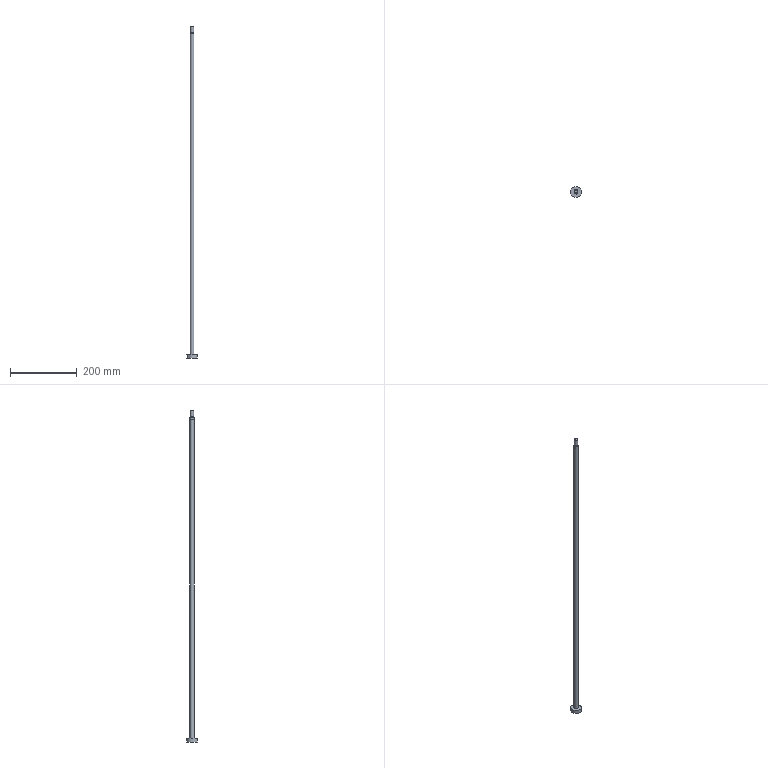Part | STEP file | 160884 CRDNG-32-400-PPV-A---(KS) | 1 solid | 19 faces | box 32 x 32 x 991.817 mm | volume 118704 mm3 | plane 9 | cylinder 4 | cone 4 | torus 2 | commonest cylinder face diameters 9.4 x1 10 x1 12 x1 32 x1
STEP:
#1=CARTESIAN_POINT('',(0.,0.,0.));
#2=DIRECTION('',(0.,0.,1.));
#3=DIRECTION('',(1.,0.,0.));
#4=AXIS2_PLACEMENT_3D('',#1,#2,#3);
#5=CARTESIAN_POINT('',(0.,4.7,226.3));
#6=VERTEX_POINT('',#5);
#7=CARTESIAN_POINT('',(4.7,0.,226.3));
#8=VERTEX_POINT('',#7);
#9=CARTESIAN_POINT('',(0.,0.,226.3));
#10=DIRECTION('',(0.,0.,1.));
#11=DIRECTION('',(0.,1.,0.));
#12=AXIS2_PLACEMENT_3D('',#9,#10,#11);
#13=CIRCLE('',#12,4.7);
#14=CARTESIAN_POINT('',(0.,0.,226.3));
#15=DIRECTION('',(0.,0.,1.));
#16=DIRECTION('',(1.,0.,0.));
#17=AXIS2_PLACEMENT_3D('',#14,#15,#16);
#18=TOROIDAL_SURFACE('',#17,5.,0.3);
#19=CARTESIAN_POINT('',(1.571,3.142));
#20=DIRECTION('',(1.,0.));
#21=VECTOR('',#20,1.);
#22=LINE('',#19,#21);
#23=(GEOMETRIC_REPRESENTATION_CONTEXT(2)PARAMETRIC_REPRESENTATION_CONTEXT()REPRESENTATION_CONTEXT('',''));
#24=DEFINITIONAL_REPRESENTATION('',(#22),#23);
#25=PCURVE('',#18,#24);
#26=CARTESIAN_POINT('',(0.,0.,226.611));
#27=DIRECTION('',(0.,0.,1.));
#28=DIRECTION('',(0.,1.,0.));
#29=AXIS2_PLACEMENT_3D('',#26,#27,#28);
#30=CYLINDRICAL_SURFACE('',#29,4.7);
#31=CARTESIAN_POINT('',(0.,-0.3105));
#32=DIRECTION('',(1.,0.));
#33=VECTOR('',#32,1.);
#34=LINE('',#31,#33);
#35=(GEOMETRIC_REPRESENTATION_CONTEXT(2)PARAMETRIC_REPRESENTATION_CONTEXT()REPRESENTATION_CONTEXT('',''));
#36=DEFINITIONAL_REPRESENTATION('',(#34),#35);
#37=PCURVE('',#30,#36);
#38=SURFACE_CURVE('',#13,(#25,#37),.PCURVE_S1.);
#39=EDGE_CURVE('',#6,#8,#38,.T.);
#40=ORIENTED_EDGE('',*,*,#39,.T.);
#41=CARTESIAN_POINT('',(5.,0.,226.));
#42=VERTEX_POINT('',#41);
#43=CARTESIAN_POINT('',(4.7,0.,226.3));
#44=CARTESIAN_POINT('',(4.7,0.,226.22));
#45=CARTESIAN_POINT('',(4.726,0.,226.142));
#46=CARTESIAN_POINT('',(4.774,0.,226.074));
#47=CARTESIAN_POINT('',(4.842,0.,226.026));
#48=CARTESIAN_POINT('',(4.92,0.,226.));
#49=CARTESIAN_POINT('',(5.,0.,226.));
#50=(BOUNDED_CURVE()B_SPLINE_CURVE(6,(#43,#44,#45,#46,#47,#48,#49),.UNSPECIFIED.,.F.,.F.)B_SPLINE_CURVE_WITH_KNOTS((7,7),(3.142,4.712),.PIECEWISE_BEZIER_KNOTS.)CURVE()GEOMETRIC_REPRESENTATION_ITEM()RATIONAL_B_SPLINE_CURVE((1.031,1.01,0.9979,0.994,0.9979,1.01,1.031))REPRESENTATION_ITEM(''));
#51=CARTESIAN_POINT('',(6.283,0.));
#52=DIRECTION('',(0.,1.));
#53=VECTOR('',#52,1.);
#54=LINE('',#51,#53);
#55=(GEOMETRIC_REPRESENTATION_CONTEXT(2)PARAMETRIC_REPRESENTATION_CONTEXT()REPRESENTATION_CONTEXT('',''));
#56=DEFINITIONAL_REPRESENTATION('',(#54),#55);
#57=PCURVE('',#18,#56);
#58=CARTESIAN_POINT('',(0.,0.));
#59=DIRECTION('',(0.,1.));
#60=VECTOR('',#59,1.);
#61=LINE('',#58,#60);
#62=(GEOMETRIC_REPRESENTATION_CONTEXT(2)PARAMETRIC_REPRESENTATION_CONTEXT()REPRESENTATION_CONTEXT('',''));
#63=DEFINITIONAL_REPRESENTATION('',(#61),#62);
#64=PCURVE('',#18,#63);
#65=SEAM_CURVE('',#50,(#57,#64),.PCURVE_S1.);
#66=EDGE_CURVE('',#8,#42,#65,.T.);
#67=ORIENTED_EDGE('',*,*,#66,.T.);
#68=CARTESIAN_POINT('',(-5.,0.,226.));
#69=VERTEX_POINT('',#68);
#70=CARTESIAN_POINT('',(0.,0.,226.));
#71=DIRECTION('',(0.,0.,1.));
#72=DIRECTION('',(1.,0.,0.));
#73=AXIS2_PLACEMENT_3D('',#70,#71,#72);
#74=CIRCLE('',#73,5.);
#75=CARTESIAN_POINT('',(0.,4.712));
#76=DIRECTION('',(1.,0.));
#77=VECTOR('',#76,1.);
#78=LINE('',#75,#77);
#79=(GEOMETRIC_REPRESENTATION_CONTEXT(2)PARAMETRIC_REPRESENTATION_CONTEXT()REPRESENTATION_CONTEXT('',''));
#80=DEFINITIONAL_REPRESENTATION('',(#78),#79);
#81=PCURVE('',#18,#80);
#82=CARTESIAN_POINT('',(0.,2.75,226.));
#83=DIRECTION('',(0.,0.,1.));
#84=DIRECTION('',(1.,0.,0.));
#85=AXIS2_PLACEMENT_3D('',#82,#83,#84);
#86=PLANE('',#85);
#87=CARTESIAN_POINT('',(0.,-2.75));
#88=DIRECTION('',(1.,0.));
#89=AXIS2_PLACEMENT_2D('',#87,#88);
#90=CIRCLE('',#89,5.);
#91=(GEOMETRIC_REPRESENTATION_CONTEXT(2)PARAMETRIC_REPRESENTATION_CONTEXT()REPRESENTATION_CONTEXT('',''));
#92=DEFINITIONAL_REPRESENTATION('',(#90),#91);
#93=PCURVE('',#86,#92);
#94=SURFACE_CURVE('',#74,(#81,#93),.PCURVE_S1.);
#95=EDGE_CURVE('',#69,#42,#94,.T.);
#96=ORIENTED_EDGE('',*,*,#95,.F.);
#97=CARTESIAN_POINT('',(0.,0.,226.));
#98=DIRECTION('',(0.,0.,1.));
#99=DIRECTION('',(1.,0.,0.));
#100=AXIS2_PLACEMENT_3D('',#97,#98,#99);
#101=CIRCLE('',#100,5.);
#102=CARTESIAN_POINT('',(0.,4.712));
#103=DIRECTION('',(1.,0.));
#104=VECTOR('',#103,1.);
#105=LINE('',#102,#104);
#106=(GEOMETRIC_REPRESENTATION_CONTEXT(2)PARAMETRIC_REPRESENTATION_CONTEXT()REPRESENTATION_CONTEXT('',''));
#107=DEFINITIONAL_REPRESENTATION('',(#105),#106);
#108=PCURVE('',#18,#107);
#109=CARTESIAN_POINT('',(0.,2.75,226.));
#110=DIRECTION('',(0.,0.,1.));
#111=DIRECTION('',(1.,0.,0.));
#112=AXIS2_PLACEMENT_3D('',#109,#110,#111);
#113=PLANE('',#112);
#114=CARTESIAN_POINT('',(0.,-2.75));
#115=DIRECTION('',(1.,0.));
#116=AXIS2_PLACEMENT_2D('',#114,#115);
#117=CIRCLE('',#116,5.);
#118=(GEOMETRIC_REPRESENTATION_CONTEXT(2)PARAMETRIC_REPRESENTATION_CONTEXT()REPRESENTATION_CONTEXT('',''));
#119=DEFINITIONAL_REPRESENTATION('',(#117),#118);
#120=PCURVE('',#113,#119);
#121=SURFACE_CURVE('',#101,(#108,#120),.PCURVE_S1.);
#122=EDGE_CURVE('',#42,#69,#121,.T.);
#123=ORIENTED_EDGE('',*,*,#122,.F.);
#124=ORIENTED_EDGE('',*,*,#66,.F.);
#125=CARTESIAN_POINT('',(0.,0.,226.3));
#126=DIRECTION('',(0.,0.,1.));
#127=DIRECTION('',(0.,1.,0.));
#128=AXIS2_PLACEMENT_3D('',#125,#126,#127);
#129=CIRCLE('',#128,4.7);
#130=CARTESIAN_POINT('',(-4.712,3.142));
#131=DIRECTION('',(1.,0.));
#132=VECTOR('',#131,1.);
#133=LINE('',#130,#132);
#134=(GEOMETRIC_REPRESENTATION_CONTEXT(2)PARAMETRIC_REPRESENTATION_CONTEXT()REPRESENTATION_CONTEXT('',''));
#135=DEFINITIONAL_REPRESENTATION('',(#133),#134);
#136=PCURVE('',#18,#135);
#137=CARTESIAN_POINT('',(0.,-0.3105));
#138=DIRECTION('',(1.,0.));
#139=VECTOR('',#138,1.);
#140=LINE('',#137,#139);
#141=(GEOMETRIC_REPRESENTATION_CONTEXT(2)PARAMETRIC_REPRESENTATION_CONTEXT()REPRESENTATION_CONTEXT('',''));
#142=DEFINITIONAL_REPRESENTATION('',(#140),#141);
#143=PCURVE('',#30,#142);
#144=SURFACE_CURVE('',#129,(#136,#143),.PCURVE_S1.);
#145=EDGE_CURVE('',#8,#6,#144,.T.);
#146=ORIENTED_EDGE('',*,*,#145,.T.);
#147=EDGE_LOOP('',(#40,#67,#96,#123,#124,#146));
#148=FACE_BOUND('',#147,.F.);
#149=ADVANCED_FACE('',(#148),#18,.F.);
#150=CARTESIAN_POINT('',(0.,4.7,226.921));
#151=VERTEX_POINT('',#150);
#152=CARTESIAN_POINT('',(0.,0.,226.921));
#153=DIRECTION('',(0.,0.,1.));
#154=DIRECTION('',(0.,1.,0.));
#155=AXIS2_PLACEMENT_3D('',#152,#153,#154);
#156=CIRCLE('',#155,4.7);
#157=CARTESIAN_POINT('',(0.,0.3105));
#158=DIRECTION('',(1.,0.));
#159=VECTOR('',#158,1.);
#160=LINE('',#157,#159);
#161=(GEOMETRIC_REPRESENTATION_CONTEXT(2)PARAMETRIC_REPRESENTATION_CONTEXT()REPRESENTATION_CONTEXT('',''));
#162=DEFINITIONAL_REPRESENTATION('',(#160),#161);
#163=PCURVE('',#30,#162);
#164=CARTESIAN_POINT('',(0.,0.,226.921));
#165=DIRECTION('',(0.,0.,1.));
#166=DIRECTION('',(1.,0.,0.));
#167=AXIS2_PLACEMENT_3D('',#164,#165,#166);
#168=TOROIDAL_SURFACE('',#167,5.3,0.6);
#169=CARTESIAN_POINT('',(1.571,9.425));
#170=DIRECTION('',(1.,0.));
#171=VECTOR('',#170,1.);
#172=LINE('',#169,#171);
#173=(GEOMETRIC_REPRESENTATION_CONTEXT(2)PARAMETRIC_REPRESENTATION_CONTEXT()REPRESENTATION_CONTEXT('',''));
#174=DEFINITIONAL_REPRESENTATION('',(#172),#173);
#175=PCURVE('',#168,#174);
#176=SURFACE_CURVE('',#156,(#163,#175),.PCURVE_S1.);
#177=EDGE_CURVE('',#151,#151,#176,.T.);
#178=ORIENTED_EDGE('',*,*,#177,.F.);
#179=CARTESIAN_POINT('',(0.,4.7,226.3));
#180=CARTESIAN_POINT('',(0.,4.7,226.921));
#181=B_SPLINE_CURVE_WITH_KNOTS('',1,(#179,#180),.UNSPECIFIED.,.F.,.F.,(2,2),(-0.3105,0.3105),.PIECEWISE_BEZIER_KNOTS.);
#182=CARTESIAN_POINT('',(0.,0.));
#183=DIRECTION('',(0.,1.));
#184=VECTOR('',#183,1.);
#185=LINE('',#182,#184);
#186=(GEOMETRIC_REPRESENTATION_CONTEXT(2)PARAMETRIC_REPRESENTATION_CONTEXT()REPRESENTATION_CONTEXT('',''));
#187=DEFINITIONAL_REPRESENTATION('',(#185),#186);
#188=PCURVE('',#30,#187);
#189=CARTESIAN_POINT('',(6.283,0.));
#190=DIRECTION('',(0.,1.));
#191=VECTOR('',#190,1.);
#192=LINE('',#189,#191);
#193=(GEOMETRIC_REPRESENTATION_CONTEXT(2)PARAMETRIC_REPRESENTATION_CONTEXT()REPRESENTATION_CONTEXT('',''));
#194=DEFINITIONAL_REPRESENTATION('',(#192),#193);
#195=PCURVE('',#30,#194);
#196=SEAM_CURVE('',#181,(#188,#195),.PCURVE_S1.);
#197=EDGE_CURVE('',#6,#151,#196,.T.);
#198=ORIENTED_EDGE('',*,*,#197,.F.);
#199=ORIENTED_EDGE('',*,*,#39,.T.);
#200=ORIENTED_EDGE('',*,*,#145,.T.);
#201=ORIENTED_EDGE('',*,*,#197,.T.);
#202=EDGE_LOOP('',(#178,#198,#199,#200,#201));
#203=FACE_BOUND('',#202,.T.);
#204=ADVANCED_FACE('',(#203),#30,.T.);
#205=CARTESIAN_POINT('',(0.,4.72,227.076));
#206=VERTEX_POINT('',#205);
#207=CARTESIAN_POINT('',(0.,0.,227.076));
#208=DIRECTION('',(0.,0.,1.));
#209=DIRECTION('',(0.,1.,0.));
#210=AXIS2_PLACEMENT_3D('',#207,#208,#209);
#211=CIRCLE('',#210,4.72);
#212=CARTESIAN_POINT('',(1.571,9.163));
#213=DIRECTION('',(1.,0.));
#214=VECTOR('',#213,1.);
#215=LINE('',#212,#214);
#216=(GEOMETRIC_REPRESENTATION_CONTEXT(2)PARAMETRIC_REPRESENTATION_CONTEXT()REPRESENTATION_CONTEXT('',''));
#217=DEFINITIONAL_REPRESENTATION('',(#215),#216);
#218=PCURVE('',#168,#217);
#219=CARTESIAN_POINT('',(0.,0.,227.598));
#220=DIRECTION('',(0.,0.,1.));
#221=DIRECTION('',(0.,1.,0.));
#222=AXIS2_PLACEMENT_3D('',#219,#220,#221);
#223=CONICAL_SURFACE('',#222,4.86,0.2618);
#224=CARTESIAN_POINT('',(0.,-0.5217));
#225=DIRECTION('',(1.,0.));
#226=VECTOR('',#225,1.);
#227=LINE('',#224,#226);
#228=(GEOMETRIC_REPRESENTATION_CONTEXT(2)PARAMETRIC_REPRESENTATION_CONTEXT()REPRESENTATION_CONTEXT('',''));
#229=DEFINITIONAL_REPRESENTATION('',(#227),#228);
#230=PCURVE('',#223,#229);
#231=SURFACE_CURVE('',#211,(#218,#230),.PCURVE_S1.);
#232=EDGE_CURVE('',#206,#206,#231,.T.);
#233=ORIENTED_EDGE('',*,*,#232,.T.);
#234=CARTESIAN_POINT('',(0.,4.72,227.076));
#235=CARTESIAN_POINT('',(0.,4.714,227.051));
#236=CARTESIAN_POINT('',(0.,4.708,227.025));
#237=CARTESIAN_POINT('',(0.,4.704,226.999));
#238=CARTESIAN_POINT('',(0.,4.701,226.973));
#239=CARTESIAN_POINT('',(0.,4.7,226.947));
#240=CARTESIAN_POINT('',(0.,4.7,226.921));
#241=(BOUNDED_CURVE()B_SPLINE_CURVE(6,(#234,#235,#236,#237,#238,#239,#240),.UNSPECIFIED.,.F.,.F.)B_SPLINE_CURVE_WITH_KNOTS((7,7),(2.88,3.142),.PIECEWISE_BEZIER_KNOTS.)CURVE()GEOMETRIC_REPRESENTATION_ITEM()RATIONAL_B_SPLINE_CURVE((1.001,1.,0.9999,0.9998,0.9999,1.,1.001))REPRESENTATION_ITEM(''));
#242=CARTESIAN_POINT('',(7.854,6.283));
#243=DIRECTION('',(0.,1.));
#244=VECTOR('',#243,1.);
#245=LINE('',#242,#244);
#246=(GEOMETRIC_REPRESENTATION_CONTEXT(2)PARAMETRIC_REPRESENTATION_CONTEXT()REPRESENTATION_CONTEXT('',''));
#247=DEFINITIONAL_REPRESENTATION('',(#245),#246);
#248=PCURVE('',#168,#247);
#249=CARTESIAN_POINT('',(1.571,6.283));
#250=DIRECTION('',(0.,1.));
#251=VECTOR('',#250,1.);
#252=LINE('',#249,#251);
#253=(GEOMETRIC_REPRESENTATION_CONTEXT(2)PARAMETRIC_REPRESENTATION_CONTEXT()REPRESENTATION_CONTEXT('',''));
#254=DEFINITIONAL_REPRESENTATION('',(#252),#253);
#255=PCURVE('',#168,#254);
#256=SEAM_CURVE('',#241,(#248,#255),.PCURVE_S1.);
#257=EDGE_CURVE('',#206,#151,#256,.T.);
#258=ORIENTED_EDGE('',*,*,#257,.T.);
#259=ORIENTED_EDGE('',*,*,#177,.F.);
#260=ORIENTED_EDGE('',*,*,#257,.F.);
#261=EDGE_LOOP('',(#233,#258,#259,#260));
#262=FACE_BOUND('',#261,.F.);
#263=ADVANCED_FACE('',(#262),#168,.F.);
#264=CARTESIAN_POINT('',(0.,5.,228.12));
#265=VERTEX_POINT('',#264);
#266=CARTESIAN_POINT('',(0.,0.,228.12));
#267=DIRECTION('',(0.,0.,1.));
#268=DIRECTION('',(0.,1.,0.));
#269=AXIS2_PLACEMENT_3D('',#266,#267,#268);
#270=CIRCLE('',#269,5.);
#271=CARTESIAN_POINT('',(0.,0.5217));
#272=DIRECTION('',(1.,0.));
#273=VECTOR('',#272,1.);
#274=LINE('',#271,#273);
#275=(GEOMETRIC_REPRESENTATION_CONTEXT(2)PARAMETRIC_REPRESENTATION_CONTEXT()REPRESENTATION_CONTEXT('',''));
#276=DEFINITIONAL_REPRESENTATION('',(#274),#275);
#277=PCURVE('',#223,#276);
#278=CARTESIAN_POINT('',(0.,0.,237.676));
#279=DIRECTION('',(0.,0.,1.));
#280=DIRECTION('',(0.,1.,0.));
#281=AXIS2_PLACEMENT_3D('',#278,#279,#280);
#282=CYLINDRICAL_SURFACE('',#281,5.);
#283=CARTESIAN_POINT('',(0.,-9.557));
#284=DIRECTION('',(1.,0.));
#285=VECTOR('',#284,1.);
#286=LINE('',#283,#285);
#287=(GEOMETRIC_REPRESENTATION_CONTEXT(2)PARAMETRIC_REPRESENTATION_CONTEXT()REPRESENTATION_CONTEXT('',''));
#288=DEFINITIONAL_REPRESENTATION('',(#286),#287);
#289=PCURVE('',#282,#288);
#290=SURFACE_CURVE('',#270,(#277,#289),.PCURVE_S1.);
#291=EDGE_CURVE('',#265,#265,#290,.T.);
#292=ORIENTED_EDGE('',*,*,#291,.F.);
#293=CARTESIAN_POINT('',(0.,4.72,227.076));
#294=CARTESIAN_POINT('',(0.,5.,228.12));
#295=B_SPLINE_CURVE_WITH_KNOTS('',1,(#293,#294),.UNSPECIFIED.,.F.,.F.,(2,2),(-0.5401,0.5401),.PIECEWISE_BEZIER_KNOTS.);
#296=CARTESIAN_POINT('',(0.,0.));
#297=DIRECTION('',(0.,1.));
#298=VECTOR('',#297,1.);
#299=LINE('',#296,#298);
#300=(GEOMETRIC_REPRESENTATION_CONTEXT(2)PARAMETRIC_REPRESENTATION_CONTEXT()REPRESENTATION_CONTEXT('',''));
#301=DEFINITIONAL_REPRESENTATION('',(#299),#300);
#302=PCURVE('',#223,#301);
#303=CARTESIAN_POINT('',(6.283,0.));
#304=DIRECTION('',(0.,1.));
#305=VECTOR('',#304,1.);
#306=LINE('',#303,#305);
#307=(GEOMETRIC_REPRESENTATION_CONTEXT(2)PARAMETRIC_REPRESENTATION_CONTEXT()REPRESENTATION_CONTEXT('',''));
#308=DEFINITIONAL_REPRESENTATION('',(#306),#307);
#309=PCURVE('',#223,#308);
#310=SEAM_CURVE('',#295,(#302,#309),.PCURVE_S1.);
#311=EDGE_CURVE('',#206,#265,#310,.T.);
#312=ORIENTED_EDGE('',*,*,#311,.F.);
#313=ORIENTED_EDGE('',*,*,#232,.T.);
#314=ORIENTED_EDGE('',*,*,#311,.T.);
#315=EDGE_LOOP('',(#292,#312,#313,#314));
#316=FACE_BOUND('',#315,.T.);
#317=ADVANCED_FACE('',(#316),#223,.T.);
#318=CARTESIAN_POINT('',(0.,5.,247.233));
#319=VERTEX_POINT('',#318);
#320=CARTESIAN_POINT('',(0.,0.,247.233));
#321=DIRECTION('',(0.,0.,1.));
#322=DIRECTION('',(0.,1.,0.));
#323=AXIS2_PLACEMENT_3D('',#320,#321,#322);
#324=CIRCLE('',#323,5.);
#325=CARTESIAN_POINT('',(0.,9.557));
#326=DIRECTION('',(1.,0.));
#327=VECTOR('',#326,1.);
#328=LINE('',#325,#327);
#329=(GEOMETRIC_REPRESENTATION_CONTEXT(2)PARAMETRIC_REPRESENTATION_CONTEXT()REPRESENTATION_CONTEXT('',''));
#330=DEFINITIONAL_REPRESENTATION('',(#328),#329);
#331=PCURVE('',#282,#330);
#332=CARTESIAN_POINT('',(0.,0.,247.617));
#333=DIRECTION('',(0.,0.,-1.));
#334=DIRECTION('',(0.,1.,0.));
#335=AXIS2_PLACEMENT_3D('',#332,#333,#334);
#336=CONICAL_SURFACE('',#335,4.617,0.7854);
#337=CARTESIAN_POINT('',(6.283,0.3835));
#338=DIRECTION('',(-1.,0.));
#339=VECTOR('',#338,1.);
#340=LINE('',#337,#339);
#341=(GEOMETRIC_REPRESENTATION_CONTEXT(2)PARAMETRIC_REPRESENTATION_CONTEXT()REPRESENTATION_CONTEXT('',''));
#342=DEFINITIONAL_REPRESENTATION('',(#340),#341);
#343=PCURVE('',#336,#342);
#344=SURFACE_CURVE('',#324,(#331,#343),.PCURVE_S1.);
#345=EDGE_CURVE('',#319,#319,#344,.T.);
#346=ORIENTED_EDGE('',*,*,#345,.F.);
#347=CARTESIAN_POINT('',(0.,5.,228.12));
#348=CARTESIAN_POINT('',(0.,5.,247.233));
#349=B_SPLINE_CURVE_WITH_KNOTS('',1,(#347,#348),.UNSPECIFIED.,.F.,.F.,(2,2),(-9.557,9.557),.PIECEWISE_BEZIER_KNOTS.);
#350=CARTESIAN_POINT('',(0.,0.));
#351=DIRECTION('',(0.,1.));
#352=VECTOR('',#351,1.);
#353=LINE('',#350,#352);
#354=(GEOMETRIC_REPRESENTATION_CONTEXT(2)PARAMETRIC_REPRESENTATION_CONTEXT()REPRESENTATION_CONTEXT('',''));
#355=DEFINITIONAL_REPRESENTATION('',(#353),#354);
#356=PCURVE('',#282,#355);
#357=CARTESIAN_POINT('',(6.283,0.));
#358=DIRECTION('',(0.,1.));
#359=VECTOR('',#358,1.);
#360=LINE('',#357,#359);
#361=(GEOMETRIC_REPRESENTATION_CONTEXT(2)PARAMETRIC_REPRESENTATION_CONTEXT()REPRESENTATION_CONTEXT('',''));
#362=DEFINITIONAL_REPRESENTATION('',(#360),#361);
#363=PCURVE('',#282,#362);
#364=SEAM_CURVE('',#349,(#356,#363),.PCURVE_S1.);
#365=EDGE_CURVE('',#265,#319,#364,.T.);
#366=ORIENTED_EDGE('',*,*,#365,.F.);
#367=ORIENTED_EDGE('',*,*,#291,.T.);
#368=ORIENTED_EDGE('',*,*,#365,.T.);
#369=EDGE_LOOP('',(#346,#366,#367,#368));
#370=FACE_BOUND('',#369,.T.);
#371=ADVANCED_FACE('',(#370),#282,.T.);
#372=CARTESIAN_POINT('',(0.,4.233,248.));
#373=VERTEX_POINT('',#372);
#374=CARTESIAN_POINT('',(0.,0.,248.));
#375=DIRECTION('',(0.,0.,1.));
#376=DIRECTION('',(0.,1.,0.));
#377=AXIS2_PLACEMENT_3D('',#374,#375,#376);
#378=CIRCLE('',#377,4.233);
#379=CARTESIAN_POINT('',(6.283,-0.3835));
#380=DIRECTION('',(-1.,0.));
#381=VECTOR('',#380,1.);
#382=LINE('',#379,#381);
#383=(GEOMETRIC_REPRESENTATION_CONTEXT(2)PARAMETRIC_REPRESENTATION_CONTEXT()REPRESENTATION_CONTEXT('',''));
#384=DEFINITIONAL_REPRESENTATION('',(#382),#383);
#385=PCURVE('',#336,#384);
#386=CARTESIAN_POINT('',(0.,2.116,248.));
#387=DIRECTION('',(0.,0.,1.));
#388=DIRECTION('',(1.,0.,0.));
#389=AXIS2_PLACEMENT_3D('',#386,#387,#388);
#390=PLANE('',#389);
#391=CARTESIAN_POINT('',(0.,-2.116));
#392=DIRECTION('',(0.,1.));
#393=AXIS2_PLACEMENT_2D('',#391,#392);
#394=CIRCLE('',#393,4.233);
#395=(GEOMETRIC_REPRESENTATION_CONTEXT(2)PARAMETRIC_REPRESENTATION_CONTEXT()REPRESENTATION_CONTEXT('',''));
#396=DEFINITIONAL_REPRESENTATION('',(#394),#395);
#397=PCURVE('',#390,#396);
#398=SURFACE_CURVE('',#378,(#385,#397),.PCURVE_S1.);
#399=EDGE_CURVE('',#373,#373,#398,.T.);
#400=ORIENTED_EDGE('',*,*,#399,.F.);
#401=CARTESIAN_POINT('',(0.,4.233,248.));
#402=CARTESIAN_POINT('',(0.,5.,247.233));
#403=B_SPLINE_CURVE_WITH_KNOTS('',1,(#401,#402),.UNSPECIFIED.,.F.,.F.,(2,2),(-0.5424,0.5424),.PIECEWISE_BEZIER_KNOTS.);
#404=CARTESIAN_POINT('',(6.283,0.));
#405=DIRECTION('',(0.,1.));
#406=VECTOR('',#405,1.);
#407=LINE('',#404,#406);
#408=(GEOMETRIC_REPRESENTATION_CONTEXT(2)PARAMETRIC_REPRESENTATION_CONTEXT()REPRESENTATION_CONTEXT('',''));
#409=DEFINITIONAL_REPRESENTATION('',(#407),#408);
#410=PCURVE('',#336,#409);
#411=CARTESIAN_POINT('',(0.,0.));
#412=DIRECTION('',(0.,1.));
#413=VECTOR('',#412,1.);
#414=LINE('',#411,#413);
#415=(GEOMETRIC_REPRESENTATION_CONTEXT(2)PARAMETRIC_REPRESENTATION_CONTEXT()REPRESENTATION_CONTEXT('',''));
#416=DEFINITIONAL_REPRESENTATION('',(#414),#415);
#417=PCURVE('',#336,#416);
#418=SEAM_CURVE('',#403,(#410,#417),.PCURVE_S1.);
#419=EDGE_CURVE('',#373,#319,#418,.T.);
#420=ORIENTED_EDGE('',*,*,#419,.T.);
#421=ORIENTED_EDGE('',*,*,#345,.T.);
#422=ORIENTED_EDGE('',*,*,#419,.F.);
#423=EDGE_LOOP('',(#400,#420,#421,#422));
#424=FACE_BOUND('',#423,.T.);
#425=ADVANCED_FACE('',(#424),#336,.T.);
#426=ORIENTED_EDGE('',*,*,#399,.T.);
#427=EDGE_LOOP('',(#426));
#428=FACE_BOUND('',#427,.T.);
#429=ADVANCED_FACE('',(#428),#390,.T.);
#430=ORIENTED_EDGE('',*,*,#122,.F.);
#431=CARTESIAN_POINT('',(5.,2.291,226.));
#432=VERTEX_POINT('',#431);
#433=CARTESIAN_POINT('',(5.,1.375,226.));
#434=DIRECTION('',(0.,1.,0.));
#435=VECTOR('',#434,1.);
#436=LINE('',#433,#435);
#437=CARTESIAN_POINT('',(5.,-1.375));
#438=DIRECTION('',(0.,1.));
#439=VECTOR('',#438,1.);
#440=LINE('',#437,#439);
#441=(GEOMETRIC_REPRESENTATION_CONTEXT(2)PARAMETRIC_REPRESENTATION_CONTEXT()REPRESENTATION_CONTEXT('',''));
#442=DEFINITIONAL_REPRESENTATION('',(#440),#441);
#443=PCURVE('',#113,#442);
#444=CARTESIAN_POINT('',(5.,0.,226.));
#445=DIRECTION('',(-1.,0.,0.));
#446=DIRECTION('',(0.,0.,1.));
#447=AXIS2_PLACEMENT_3D('',#444,#445,#446);
#448=PLANE('',#447);
#449=CARTESIAN_POINT('',(0.,1.375));
#450=DIRECTION('',(0.,1.));
#451=VECTOR('',#450,1.);
#452=LINE('',#449,#451);
#453=(GEOMETRIC_REPRESENTATION_CONTEXT(2)PARAMETRIC_REPRESENTATION_CONTEXT()REPRESENTATION_CONTEXT('',''));
#454=DEFINITIONAL_REPRESENTATION('',(#452),#453);
#455=PCURVE('',#448,#454);
#456=SURFACE_CURVE('',#436,(#443,#455),.PCURVE_S1.);
#457=EDGE_CURVE('',#42,#432,#456,.T.);
#458=ORIENTED_EDGE('',*,*,#457,.T.);
#459=CARTESIAN_POINT('',(-5.,2.291,226.));
#460=VERTEX_POINT('',#459);
#461=CARTESIAN_POINT('',(0.,0.,226.));
#462=DIRECTION('',(0.,0.,1.));
#463=DIRECTION('',(0.,1.,0.));
#464=AXIS2_PLACEMENT_3D('',#461,#462,#463);
#465=CIRCLE('',#464,5.5);
#466=CARTESIAN_POINT('',(0.,-2.75));
#467=DIRECTION('',(0.,1.));
#468=AXIS2_PLACEMENT_2D('',#466,#467);
#469=CIRCLE('',#468,5.5);
#470=(GEOMETRIC_REPRESENTATION_CONTEXT(2)PARAMETRIC_REPRESENTATION_CONTEXT()REPRESENTATION_CONTEXT('',''));
#471=DEFINITIONAL_REPRESENTATION('',(#469),#470);
#472=PCURVE('',#113,#471);
#473=CARTESIAN_POINT('',(0.,0.,225.75));
#474=DIRECTION('',(0.,0.,-1.));
#475=DIRECTION('',(0.,1.,0.));
#476=AXIS2_PLACEMENT_3D('',#473,#474,#475);
#477=CONICAL_SURFACE('',#476,5.75,0.7854);
#478=CARTESIAN_POINT('',(12.566,-0.25));
#479=DIRECTION('',(-1.,0.));
#480=VECTOR('',#479,1.);
#481=LINE('',#478,#480);
#482=(GEOMETRIC_REPRESENTATION_CONTEXT(2)PARAMETRIC_REPRESENTATION_CONTEXT()REPRESENTATION_CONTEXT('',''));
#483=DEFINITIONAL_REPRESENTATION('',(#481),#482);
#484=PCURVE('',#477,#483);
#485=SURFACE_CURVE('',#465,(#472,#484),.PCURVE_S1.);
#486=EDGE_CURVE('',#432,#460,#485,.T.);
#487=ORIENTED_EDGE('',*,*,#486,.T.);
#488=CARTESIAN_POINT('',(-5.,1.375,226.));
#489=DIRECTION('',(0.,-1.,0.));
#490=VECTOR('',#489,1.);
#491=LINE('',#488,#490);
#492=CARTESIAN_POINT('',(-5.,-1.375));
#493=DIRECTION('',(0.,-1.));
#494=VECTOR('',#493,1.);
#495=LINE('',#492,#494);
#496=(GEOMETRIC_REPRESENTATION_CONTEXT(2)PARAMETRIC_REPRESENTATION_CONTEXT()REPRESENTATION_CONTEXT('',''));
#497=DEFINITIONAL_REPRESENTATION('',(#495),#496);
#498=PCURVE('',#113,#497);
#499=CARTESIAN_POINT('',(-5.,0.,220.));
#500=DIRECTION('',(1.,0.,0.));
#501=DIRECTION('',(0.,0.,-1.));
#502=AXIS2_PLACEMENT_3D('',#499,#500,#501);
#503=PLANE('',#502);
#504=CARTESIAN_POINT('',(-6.,1.375));
#505=DIRECTION('',(0.,-1.));
#506=VECTOR('',#505,1.);
#507=LINE('',#504,#506);
#508=(GEOMETRIC_REPRESENTATION_CONTEXT(2)PARAMETRIC_REPRESENTATION_CONTEXT()REPRESENTATION_CONTEXT('',''));
#509=DEFINITIONAL_REPRESENTATION('',(#507),#508);
#510=PCURVE('',#503,#509);
#511=SURFACE_CURVE('',#491,(#498,#510),.PCURVE_S1.);
#512=EDGE_CURVE('',#460,#69,#511,.T.);
#513=ORIENTED_EDGE('',*,*,#512,.T.);
#514=EDGE_LOOP('',(#430,#458,#487,#513));
#515=FACE_BOUND('',#514,.T.);
#516=ADVANCED_FACE('',(#515),#113,.T.);
#517=ORIENTED_EDGE('',*,*,#95,.F.);
#518=CARTESIAN_POINT('',(-5.,-2.291,226.));
#519=VERTEX_POINT('',#518);
#520=CARTESIAN_POINT('',(-5.,1.375,226.));
#521=DIRECTION('',(0.,-1.,0.));
#522=VECTOR('',#521,1.);
#523=LINE('',#520,#522);
#524=CARTESIAN_POINT('',(-5.,-1.375));
#525=DIRECTION('',(0.,-1.));
#526=VECTOR('',#525,1.);
#527=LINE('',#524,#526);
#528=(GEOMETRIC_REPRESENTATION_CONTEXT(2)PARAMETRIC_REPRESENTATION_CONTEXT()REPRESENTATION_CONTEXT('',''));
#529=DEFINITIONAL_REPRESENTATION('',(#527),#528);
#530=PCURVE('',#86,#529);
#531=CARTESIAN_POINT('',(-6.,1.375));
#532=DIRECTION('',(0.,-1.));
#533=VECTOR('',#532,1.);
#534=LINE('',#531,#533);
#535=(GEOMETRIC_REPRESENTATION_CONTEXT(2)PARAMETRIC_REPRESENTATION_CONTEXT()REPRESENTATION_CONTEXT('',''));
#536=DEFINITIONAL_REPRESENTATION('',(#534),#535);
#537=PCURVE('',#503,#536);
#538=SURFACE_CURVE('',#523,(#530,#537),.PCURVE_S1.);
#539=EDGE_CURVE('',#69,#519,#538,.T.);
#540=ORIENTED_EDGE('',*,*,#539,.T.);
#541=CARTESIAN_POINT('',(5.,-2.291,226.));
#542=VERTEX_POINT('',#541);
#543=CARTESIAN_POINT('',(0.,0.,226.));
#544=DIRECTION('',(0.,0.,1.));
#545=DIRECTION('',(0.,1.,0.));
#546=AXIS2_PLACEMENT_3D('',#543,#544,#545);
#547=CIRCLE('',#546,5.5);
#548=CARTESIAN_POINT('',(0.,-2.75));
#549=DIRECTION('',(0.,1.));
#550=AXIS2_PLACEMENT_2D('',#548,#549);
#551=CIRCLE('',#550,5.5);
#552=(GEOMETRIC_REPRESENTATION_CONTEXT(2)PARAMETRIC_REPRESENTATION_CONTEXT()REPRESENTATION_CONTEXT('',''));
#553=DEFINITIONAL_REPRESENTATION('',(#551),#552);
#554=PCURVE('',#86,#553);
#555=CARTESIAN_POINT('',(0.,0.,225.75));
#556=DIRECTION('',(0.,0.,-1.));
#557=DIRECTION('',(0.,1.,0.));
#558=AXIS2_PLACEMENT_3D('',#555,#556,#557);
#559=CONICAL_SURFACE('',#558,5.75,0.7854);
#560=CARTESIAN_POINT('',(6.283,-0.25));
#561=DIRECTION('',(-1.,0.));
#562=VECTOR('',#561,1.);
#563=LINE('',#560,#562);
#564=(GEOMETRIC_REPRESENTATION_CONTEXT(2)PARAMETRIC_REPRESENTATION_CONTEXT()REPRESENTATION_CONTEXT('',''));
#565=DEFINITIONAL_REPRESENTATION('',(#563),#564);
#566=PCURVE('',#559,#565);
#567=SURFACE_CURVE('',#547,(#554,#566),.PCURVE_S1.);
#568=EDGE_CURVE('',#519,#542,#567,.T.);
#569=ORIENTED_EDGE('',*,*,#568,.T.);
#570=CARTESIAN_POINT('',(5.,1.375,226.));
#571=DIRECTION('',(0.,1.,0.));
#572=VECTOR('',#571,1.);
#573=LINE('',#570,#572);
#574=CARTESIAN_POINT('',(5.,-1.375));
#575=DIRECTION('',(0.,1.));
#576=VECTOR('',#575,1.);
#577=LINE('',#574,#576);
#578=(GEOMETRIC_REPRESENTATION_CONTEXT(2)PARAMETRIC_REPRESENTATION_CONTEXT()REPRESENTATION_CONTEXT('',''));
#579=DEFINITIONAL_REPRESENTATION('',(#577),#578);
#580=PCURVE('',#86,#579);
#581=CARTESIAN_POINT('',(0.,1.375));
#582=DIRECTION('',(0.,1.));
#583=VECTOR('',#582,1.);
#584=LINE('',#581,#583);
#585=(GEOMETRIC_REPRESENTATION_CONTEXT(2)PARAMETRIC_REPRESENTATION_CONTEXT()REPRESENTATION_CONTEXT('',''));
#586=DEFINITIONAL_REPRESENTATION('',(#584),#585);
#587=PCURVE('',#448,#586);
#588=SURFACE_CURVE('',#573,(#580,#587),.PCURVE_S1.);
#589=EDGE_CURVE('',#542,#42,#588,.T.);
#590=ORIENTED_EDGE('',*,*,#589,.T.);
#591=EDGE_LOOP('',(#517,#540,#569,#590));
#592=FACE_BOUND('',#591,.T.);
#593=ADVANCED_FACE('',(#592),#86,.T.);
#594=CARTESIAN_POINT('',(-5.,3.317,220.));
#595=VERTEX_POINT('',#594);
#596=CARTESIAN_POINT('',(-5.,3.317,225.5));
#597=VERTEX_POINT('',#596);
#598=CARTESIAN_POINT('',(-5.,3.317,-303.825));
#599=DIRECTION('',(0.,0.,1.));
#600=VECTOR('',#599,1.);
#601=LINE('',#598,#600);
#602=CARTESIAN_POINT('',(523.825,3.317));
#603=DIRECTION('',(-1.,0.));
#604=VECTOR('',#603,1.);
#605=LINE('',#602,#604);
#606=(GEOMETRIC_REPRESENTATION_CONTEXT(2)PARAMETRIC_REPRESENTATION_CONTEXT()REPRESENTATION_CONTEXT('',''));
#607=DEFINITIONAL_REPRESENTATION('',(#605),#606);
#608=PCURVE('',#503,#607);
#609=CARTESIAN_POINT('',(0.,0.,-303.825));
#610=DIRECTION('',(0.,0.,1.));
#611=DIRECTION('',(0.,1.,0.));
#612=AXIS2_PLACEMENT_3D('',#609,#610,#611);
#613=CYLINDRICAL_SURFACE('',#612,6.);
#614=CARTESIAN_POINT('',(7.268,0.));
#615=DIRECTION('',(0.,1.));
#616=VECTOR('',#615,1.);
#617=LINE('',#614,#616);
#618=(GEOMETRIC_REPRESENTATION_CONTEXT(2)PARAMETRIC_REPRESENTATION_CONTEXT()REPRESENTATION_CONTEXT('',''));
#619=DEFINITIONAL_REPRESENTATION('',(#617),#618);
#620=PCURVE('',#613,#619);
#621=SURFACE_CURVE('',#601,(#608,#620),.PCURVE_S1.);
#622=EDGE_CURVE('',#595,#597,#621,.T.);
#623=ORIENTED_EDGE('',*,*,#622,.F.);
#624=CARTESIAN_POINT('',(-5.,-3.317,220.));
#625=VERTEX_POINT('',#624);
#626=CARTESIAN_POINT('',(-5.,0.,220.));
#627=DIRECTION('',(0.,1.,0.));
#628=VECTOR('',#627,1.);
#629=LINE('',#626,#628);
#630=CARTESIAN_POINT('',(0.,0.));
#631=DIRECTION('',(0.,1.));
#632=VECTOR('',#631,1.);
#633=LINE('',#630,#632);
#634=(GEOMETRIC_REPRESENTATION_CONTEXT(2)PARAMETRIC_REPRESENTATION_CONTEXT()REPRESENTATION_CONTEXT('',''));
#635=DEFINITIONAL_REPRESENTATION('',(#633),#634);
#636=PCURVE('',#503,#635);
#637=CARTESIAN_POINT('',(-15.,0.,220.));
#638=DIRECTION('',(0.,0.,-1.));
#639=DIRECTION('',(-1.,0.,0.));
#640=AXIS2_PLACEMENT_3D('',#637,#638,#639);
#641=PLANE('',#640);
#642=CARTESIAN_POINT('',(-10.,0.));
#643=DIRECTION('',(0.,1.));
#644=VECTOR('',#643,1.);
#645=LINE('',#642,#644);
#646=(GEOMETRIC_REPRESENTATION_CONTEXT(2)PARAMETRIC_REPRESENTATION_CONTEXT()REPRESENTATION_CONTEXT('',''));
#647=DEFINITIONAL_REPRESENTATION('',(#645),#646);
#648=PCURVE('',#641,#647);
#649=SURFACE_CURVE('',#629,(#636,#648),.PCURVE_S1.);
#650=EDGE_CURVE('',#625,#595,#649,.T.);
#651=ORIENTED_EDGE('',*,*,#650,.F.);
#652=CARTESIAN_POINT('',(-5.,-3.317,225.5));
#653=VERTEX_POINT('',#652);
#654=CARTESIAN_POINT('',(-5.,-3.317,-303.825));
#655=DIRECTION('',(0.,0.,-1.));
#656=VECTOR('',#655,1.);
#657=LINE('',#654,#656);
#658=CARTESIAN_POINT('',(523.825,-3.317));
#659=DIRECTION('',(1.,0.));
#660=VECTOR('',#659,1.);
#661=LINE('',#658,#660);
#662=(GEOMETRIC_REPRESENTATION_CONTEXT(2)PARAMETRIC_REPRESENTATION_CONTEXT()REPRESENTATION_CONTEXT('',''));
#663=DEFINITIONAL_REPRESENTATION('',(#661),#662);
#664=PCURVE('',#503,#663);
#665=CARTESIAN_POINT('',(2.156,0.));
#666=DIRECTION('',(0.,-1.));
#667=VECTOR('',#666,1.);
#668=LINE('',#665,#667);
#669=(GEOMETRIC_REPRESENTATION_CONTEXT(2)PARAMETRIC_REPRESENTATION_CONTEXT()REPRESENTATION_CONTEXT('',''));
#670=DEFINITIONAL_REPRESENTATION('',(#668),#669);
#671=PCURVE('',#613,#670);
#672=SURFACE_CURVE('',#657,(#664,#671),.PCURVE_S1.);
#673=EDGE_CURVE('',#653,#625,#672,.T.);
#674=ORIENTED_EDGE('',*,*,#673,.F.);
#675=CARTESIAN_POINT('',(-5.,-3.317,225.5));
#676=CARTESIAN_POINT('',(-5.,-2.782,225.796));
#677=CARTESIAN_POINT('',(-5.,-2.291,226.));
#678=(BOUNDED_CURVE()B_SPLINE_CURVE(2,(#675,#676,#677),.UNSPECIFIED.,.F.,.F.)B_SPLINE_CURVE_WITH_KNOTS((3,3),(9880.773,11059.121),.PIECEWISE_BEZIER_KNOTS.)CURVE()GEOMETRIC_REPRESENTATION_ITEM()RATIONAL_B_SPLINE_CURVE((9094.227,9345.458,9527.285))REPRESENTATION_ITEM(''));
#679=CARTESIAN_POINT('',(-5.5,-3.317));
#680=CARTESIAN_POINT('',(-5.796,-2.782));
#681=CARTESIAN_POINT('',(-6.,-2.291));
#682=(BOUNDED_CURVE()B_SPLINE_CURVE(2,(#679,#680,#681),.UNSPECIFIED.,.F.,.F.)B_SPLINE_CURVE_WITH_KNOTS((3,3),(9880.773,11059.121),.PIECEWISE_BEZIER_KNOTS.)CURVE()GEOMETRIC_REPRESENTATION_ITEM()RATIONAL_B_SPLINE_CURVE((9094.227,9345.458,9527.285))REPRESENTATION_ITEM(''));
#683=(GEOMETRIC_REPRESENTATION_CONTEXT(2)PARAMETRIC_REPRESENTATION_CONTEXT()REPRESENTATION_CONTEXT('',''));
#684=DEFINITIONAL_REPRESENTATION('',(#682),#683);
#685=PCURVE('',#503,#684);
#686=CARTESIAN_POINT('',(4.127,0.25));
#687=CARTESIAN_POINT('',(4.129,0.2408));
#688=CARTESIAN_POINT('',(4.134,0.2225));
#689=CARTESIAN_POINT('',(4.141,0.1956));
#690=CARTESIAN_POINT('',(4.148,0.1692));
#691=CARTESIAN_POINT('',(4.155,0.1432));
#692=CARTESIAN_POINT('',(4.162,0.1177));
#693=CARTESIAN_POINT('',(4.169,0.0927));
#694=CARTESIAN_POINT('',(4.176,0.0681));
#695=CARTESIAN_POINT('',(4.183,0.04395));
#696=CARTESIAN_POINT('',(4.19,0.02025));
#697=CARTESIAN_POINT('',(4.197,-0.003026));
#698=CARTESIAN_POINT('',(4.204,-0.02587));
#699=CARTESIAN_POINT('',(4.211,-0.04829));
#700=CARTESIAN_POINT('',(4.218,-0.07029));
#701=CARTESIAN_POINT('',(4.225,-0.09187));
#702=CARTESIAN_POINT('',(4.232,-0.113));
#703=CARTESIAN_POINT('',(4.24,-0.1338));
#704=CARTESIAN_POINT('',(4.247,-0.1542));
#705=CARTESIAN_POINT('',(4.254,-0.1741));
#706=CARTESIAN_POINT('',(4.261,-0.1937));
#707=CARTESIAN_POINT('',(4.268,-0.2129));
#708=CARTESIAN_POINT('',(4.275,-0.2317));
#709=CARTESIAN_POINT('',(4.28,-0.2439));
#710=CARTESIAN_POINT('',(4.283,-0.25));
#711=B_SPLINE_CURVE_WITH_KNOTS('',3,(#686,#687,#688,#689,#690,#691,#692,#693,#694,#695,#696,#697,#698,#699,#700,#701,#702,#703,#704,#705,#706,#707,#708,#709,#710),.UNSPECIFIED.,.F.,.F.,(4,1,1,1,1,1,1,1,1,1,1,1,1,1,1,1,1,1,1,1,1,1,4),(9880.773,9934.334,9987.895,10041.457,10095.018,10148.579,10202.14,10255.702,10309.263,10362.824,10416.385,10469.947,10523.508,10577.069,10630.631,10684.192,10737.753,10791.314,10844.876,10898.437,10951.998,11005.559,11059.121),.QUASI_UNIFORM_KNOTS.);
#712=(GEOMETRIC_REPRESENTATION_CONTEXT(2)PARAMETRIC_REPRESENTATION_CONTEXT()REPRESENTATION_CONTEXT('',''));
#713=DEFINITIONAL_REPRESENTATION('',(#711),#712);
#714=PCURVE('',#559,#713);
#715=SURFACE_CURVE('',#678,(#685,#714),.PCURVE_S1.);
#716=EDGE_CURVE('',#653,#519,#715,.T.);
#717=ORIENTED_EDGE('',*,*,#716,.T.);
#718=ORIENTED_EDGE('',*,*,#539,.F.);
#719=ORIENTED_EDGE('',*,*,#512,.F.);
#720=CARTESIAN_POINT('',(-5.,2.291,226.));
#721=CARTESIAN_POINT('',(-5.,2.572,225.883));
#722=CARTESIAN_POINT('',(-5.,3.087,225.627));
#723=CARTESIAN_POINT('',(-5.,3.317,225.5));
#724=(BOUNDED_CURVE()B_SPLINE_CURVE(2,(#720,#721,#722,#723),.UNSPECIFIED.,.F.,.F.)B_SPLINE_CURVE_WITH_KNOTS((3,1,3),(17233.353,17914.392,18411.701),.UNSPECIFIED.)CURVE()GEOMETRIC_REPRESENTATION_ITEM()RATIONAL_B_SPLINE_CURVE((9527.285,9422.196,9200.256,9094.227))REPRESENTATION_ITEM(''));
#725=CARTESIAN_POINT('',(-6.,2.291));
#726=CARTESIAN_POINT('',(-5.883,2.572));
#727=CARTESIAN_POINT('',(-5.627,3.087));
#728=CARTESIAN_POINT('',(-5.5,3.317));
#729=(BOUNDED_CURVE()B_SPLINE_CURVE(2,(#725,#726,#727,#728),.UNSPECIFIED.,.F.,.F.)B_SPLINE_CURVE_WITH_KNOTS((3,1,3),(17233.353,17914.392,18411.701),.UNSPECIFIED.)CURVE()GEOMETRIC_REPRESENTATION_ITEM()RATIONAL_B_SPLINE_CURVE((9527.285,9422.196,9200.256,9094.227))REPRESENTATION_ITEM(''));
#730=(GEOMETRIC_REPRESENTATION_CONTEXT(2)PARAMETRIC_REPRESENTATION_CONTEXT()REPRESENTATION_CONTEXT('',''));
#731=DEFINITIONAL_REPRESENTATION('',(#729),#730);
#732=PCURVE('',#503,#731);
#733=CARTESIAN_POINT('',(5.142,-0.25));
#734=CARTESIAN_POINT('',(5.144,-0.2439));
#735=CARTESIAN_POINT('',(5.149,-0.2317));
#736=CARTESIAN_POINT('',(5.157,-0.2129));
#737=CARTESIAN_POINT('',(5.164,-0.1937));
#738=CARTESIAN_POINT('',(5.171,-0.1741));
#739=CARTESIAN_POINT('',(5.178,-0.1542));
#740=CARTESIAN_POINT('',(5.185,-0.1338));
#741=CARTESIAN_POINT('',(5.192,-0.113));
#742=CARTESIAN_POINT('',(5.2,-0.09187));
#743=CARTESIAN_POINT('',(5.207,-0.07029));
#744=CARTESIAN_POINT('',(5.214,-0.04829));
#745=CARTESIAN_POINT('',(5.221,-0.02587));
#746=CARTESIAN_POINT('',(5.228,-0.003026));
#747=CARTESIAN_POINT('',(5.235,0.02025));
#748=CARTESIAN_POINT('',(5.242,0.04395));
#749=CARTESIAN_POINT('',(5.249,0.0681));
#750=CARTESIAN_POINT('',(5.256,0.0927));
#751=CARTESIAN_POINT('',(5.263,0.1177));
#752=CARTESIAN_POINT('',(5.27,0.1432));
#753=CARTESIAN_POINT('',(5.277,0.1692));
#754=CARTESIAN_POINT('',(5.284,0.1956));
#755=CARTESIAN_POINT('',(5.291,0.2225));
#756=CARTESIAN_POINT('',(5.296,0.2408));
#757=CARTESIAN_POINT('',(5.298,0.25));
#758=B_SPLINE_CURVE_WITH_KNOTS('',3,(#733,#734,#735,#736,#737,#738,#739,#740,#741,#742,#743,#744,#745,#746,#747,#748,#749,#750,#751,#752,#753,#754,#755,#756,#757),.UNSPECIFIED.,.F.,.F.,(4,1,1,1,1,1,1,1,1,1,1,1,1,1,1,1,1,1,1,1,1,1,4),(17233.353,17286.914,17340.476,17394.037,17447.598,17501.159,17554.721,17608.282,17661.843,17715.404,17768.966,17822.527,17876.088,17929.649,17983.211,18036.772,18090.333,18143.895,18197.456,18251.017,18304.578,18358.14,18411.701),.QUASI_UNIFORM_KNOTS.);
#759=(GEOMETRIC_REPRESENTATION_CONTEXT(2)PARAMETRIC_REPRESENTATION_CONTEXT()REPRESENTATION_CONTEXT('',''));
#760=DEFINITIONAL_REPRESENTATION('',(#758),#759);
#761=PCURVE('',#477,#760);
#762=SURFACE_CURVE('',#724,(#732,#761),.PCURVE_S1.);
#763=EDGE_CURVE('',#460,#597,#762,.T.);
#764=ORIENTED_EDGE('',*,*,#763,.T.);
#765=EDGE_LOOP('',(#623,#651,#674,#717,#718,#719,#764));
#766=FACE_BOUND('',#765,.T.);
#767=ADVANCED_FACE('',(#766),#503,.F.);
#768=CARTESIAN_POINT('',(5.,3.317,225.5));
#769=VERTEX_POINT('',#768);
#770=CARTESIAN_POINT('',(5.,3.317,225.5));
#771=CARTESIAN_POINT('',(5.,2.782,225.796));
#772=CARTESIAN_POINT('',(5.,2.291,226.));
#773=(BOUNDED_CURVE()B_SPLINE_CURVE(2,(#770,#771,#772),.UNSPECIFIED.,.F.,.F.)B_SPLINE_CURVE_WITH_KNOTS((3,3),(9880.773,11059.121),.PIECEWISE_BEZIER_KNOTS.)CURVE()GEOMETRIC_REPRESENTATION_ITEM()RATIONAL_B_SPLINE_CURVE((9094.227,9345.458,9527.285))REPRESENTATION_ITEM(''));
#774=CARTESIAN_POINT('',(-0.5,3.317));
#775=CARTESIAN_POINT('',(-0.2043,2.782));
#776=CARTESIAN_POINT('',(0.00000001,2.291));
#777=(BOUNDED_CURVE()B_SPLINE_CURVE(2,(#774,#775,#776),.UNSPECIFIED.,.F.,.F.)B_SPLINE_CURVE_WITH_KNOTS((3,3),(9880.773,11059.121),.PIECEWISE_BEZIER_KNOTS.)CURVE()GEOMETRIC_REPRESENTATION_ITEM()RATIONAL_B_SPLINE_CURVE((9094.227,9345.458,9527.285))REPRESENTATION_ITEM(''));
#778=(GEOMETRIC_REPRESENTATION_CONTEXT(2)PARAMETRIC_REPRESENTATION_CONTEXT()REPRESENTATION_CONTEXT('',''));
#779=DEFINITIONAL_REPRESENTATION('',(#777),#778);
#780=PCURVE('',#448,#779);
#781=CARTESIAN_POINT('',(7.268,0.25));
#782=CARTESIAN_POINT('',(7.271,0.2408));
#783=CARTESIAN_POINT('',(7.275,0.2225));
#784=CARTESIAN_POINT('',(7.282,0.1956));
#785=CARTESIAN_POINT('',(7.289,0.1692));
#786=CARTESIAN_POINT('',(7.296,0.1432));
#787=CARTESIAN_POINT('',(7.303,0.1177));
#788=CARTESIAN_POINT('',(7.31,0.0927));
#789=CARTESIAN_POINT('',(7.317,0.0681));
#790=CARTESIAN_POINT('',(7.324,0.04395));
#791=CARTESIAN_POINT('',(7.331,0.02025));
#792=CARTESIAN_POINT('',(7.338,-0.003026));
#793=CARTESIAN_POINT('',(7.345,-0.02587));
#794=CARTESIAN_POINT('',(7.353,-0.04829));
#795=CARTESIAN_POINT('',(7.36,-0.07029));
#796=CARTESIAN_POINT('',(7.367,-0.09187));
#797=CARTESIAN_POINT('',(7.374,-0.113));
#798=CARTESIAN_POINT('',(7.381,-0.1338));
#799=CARTESIAN_POINT('',(7.388,-0.1542));
#800=CARTESIAN_POINT('',(7.395,-0.1741));
#801=CARTESIAN_POINT('',(7.403,-0.1937));
#802=CARTESIAN_POINT('',(7.41,-0.2129));
#803=CARTESIAN_POINT('',(7.417,-0.2317));
#804=CARTESIAN_POINT('',(7.422,-0.2439));
#805=CARTESIAN_POINT('',(7.424,-0.25));
#806=B_SPLINE_CURVE_WITH_KNOTS('',3,(#781,#782,#783,#784,#785,#786,#787,#788,#789,#790,#791,#792,#793,#794,#795,#796,#797,#798,#799,#800,#801,#802,#803,#804,#805),.UNSPECIFIED.,.F.,.F.,(4,1,1,1,1,1,1,1,1,1,1,1,1,1,1,1,1,1,1,1,1,1,4),(9880.773,9934.334,9987.895,10041.457,10095.018,10148.579,10202.14,10255.702,10309.263,10362.824,10416.385,10469.947,10523.508,10577.069,10630.631,10684.192,10737.753,10791.314,10844.876,10898.437,10951.998,11005.559,11059.121),.QUASI_UNIFORM_KNOTS.);
#807=(GEOMETRIC_REPRESENTATION_CONTEXT(2)PARAMETRIC_REPRESENTATION_CONTEXT()REPRESENTATION_CONTEXT('',''));
#808=DEFINITIONAL_REPRESENTATION('',(#806),#807);
#809=PCURVE('',#477,#808);
#810=SURFACE_CURVE('',#773,(#780,#809),.PCURVE_S1.);
#811=EDGE_CURVE('',#769,#432,#810,.T.);
#812=ORIENTED_EDGE('',*,*,#811,.T.);
#813=ORIENTED_EDGE('',*,*,#457,.F.);
#814=ORIENTED_EDGE('',*,*,#589,.F.);
#815=CARTESIAN_POINT('',(5.,-3.317,225.5));
#816=VERTEX_POINT('',#815);
#817=CARTESIAN_POINT('',(5.,-2.291,226.));
#818=CARTESIAN_POINT('',(5.,-2.572,225.883));
#819=CARTESIAN_POINT('',(5.,-3.087,225.627));
#820=CARTESIAN_POINT('',(5.,-3.317,225.5));
#821=(BOUNDED_CURVE()B_SPLINE_CURVE(2,(#817,#818,#819,#820),.UNSPECIFIED.,.F.,.F.)B_SPLINE_CURVE_WITH_KNOTS((3,1,3),(17233.353,17914.392,18411.701),.UNSPECIFIED.)CURVE()GEOMETRIC_REPRESENTATION_ITEM()RATIONAL_B_SPLINE_CURVE((9527.285,9422.196,9200.256,9094.227))REPRESENTATION_ITEM(''));
#822=CARTESIAN_POINT('',(0.00000001,-2.291));
#823=CARTESIAN_POINT('',(-0.1171,-2.572));
#824=CARTESIAN_POINT('',(-0.3732,-3.087));
#825=CARTESIAN_POINT('',(-0.5,-3.317));
#826=(BOUNDED_CURVE()B_SPLINE_CURVE(2,(#822,#823,#824,#825),.UNSPECIFIED.,.F.,.F.)B_SPLINE_CURVE_WITH_KNOTS((3,1,3),(17233.353,17914.392,18411.701),.UNSPECIFIED.)CURVE()GEOMETRIC_REPRESENTATION_ITEM()RATIONAL_B_SPLINE_CURVE((9527.285,9422.196,9200.256,9094.227))REPRESENTATION_ITEM(''));
#827=(GEOMETRIC_REPRESENTATION_CONTEXT(2)PARAMETRIC_REPRESENTATION_CONTEXT()REPRESENTATION_CONTEXT('',''));
#828=DEFINITIONAL_REPRESENTATION('',(#826),#827);
#829=PCURVE('',#448,#828);
#830=CARTESIAN_POINT('',(2.,-0.25));
#831=CARTESIAN_POINT('',(2.003,-0.2439));
#832=CARTESIAN_POINT('',(2.008,-0.2317));
#833=CARTESIAN_POINT('',(2.015,-0.2129));
#834=CARTESIAN_POINT('',(2.022,-0.1937));
#835=CARTESIAN_POINT('',(2.029,-0.1741));
#836=CARTESIAN_POINT('',(2.036,-0.1542));
#837=CARTESIAN_POINT('',(2.044,-0.1338));
#838=CARTESIAN_POINT('',(2.051,-0.113));
#839=CARTESIAN_POINT('',(2.058,-0.09187));
#840=CARTESIAN_POINT('',(2.065,-0.07029));
#841=CARTESIAN_POINT('',(2.072,-0.04829));
#842=CARTESIAN_POINT('',(2.079,-0.02587));
#843=CARTESIAN_POINT('',(2.086,-0.003026));
#844=CARTESIAN_POINT('',(2.093,0.02025));
#845=CARTESIAN_POINT('',(2.101,0.04395));
#846=CARTESIAN_POINT('',(2.108,0.0681));
#847=CARTESIAN_POINT('',(2.115,0.0927));
#848=CARTESIAN_POINT('',(2.122,0.1177));
#849=CARTESIAN_POINT('',(2.129,0.1432));
#850=CARTESIAN_POINT('',(2.136,0.1692));
#851=CARTESIAN_POINT('',(2.143,0.1956));
#852=CARTESIAN_POINT('',(2.15,0.2225));
#853=CARTESIAN_POINT('',(2.154,0.2408));
#854=CARTESIAN_POINT('',(2.156,0.25));
#855=B_SPLINE_CURVE_WITH_KNOTS('',3,(#830,#831,#832,#833,#834,#835,#836,#837,#838,#839,#840,#841,#842,#843,#844,#845,#846,#847,#848,#849,#850,#851,#852,#853,#854),.UNSPECIFIED.,.F.,.F.,(4,1,1,1,1,1,1,1,1,1,1,1,1,1,1,1,1,1,1,1,1,1,4),(17233.353,17286.914,17340.476,17394.037,17447.598,17501.159,17554.721,17608.282,17661.843,17715.404,17768.966,17822.527,17876.088,17929.649,17983.211,18036.772,18090.333,18143.895,18197.456,18251.017,18304.578,18358.14,18411.701),.QUASI_UNIFORM_KNOTS.);
#856=(GEOMETRIC_REPRESENTATION_CONTEXT(2)PARAMETRIC_REPRESENTATION_CONTEXT()REPRESENTATION_CONTEXT('',''));
#857=DEFINITIONAL_REPRESENTATION('',(#855),#856);
#858=PCURVE('',#559,#857);
#859=SURFACE_CURVE('',#821,(#829,#858),.PCURVE_S1.);
#860=EDGE_CURVE('',#542,#816,#859,.T.);
#861=ORIENTED_EDGE('',*,*,#860,.T.);
#862=CARTESIAN_POINT('',(5.,-3.317,220.));
#863=VERTEX_POINT('',#862);
#864=CARTESIAN_POINT('',(5.,-3.317,-303.825));
#865=DIRECTION('',(0.,0.,1.));
#866=VECTOR('',#865,1.);
#867=LINE('',#864,#866);
#868=CARTESIAN_POINT('',(-529.825,-3.317));
#869=DIRECTION('',(1.,0.));
#870=VECTOR('',#869,1.);
#871=LINE('',#868,#870);
#872=(GEOMETRIC_REPRESENTATION_CONTEXT(2)PARAMETRIC_REPRESENTATION_CONTEXT()REPRESENTATION_CONTEXT('',''));
#873=DEFINITIONAL_REPRESENTATION('',(#871),#872);
#874=PCURVE('',#448,#873);
#875=CARTESIAN_POINT('',(4.127,0.));
#876=DIRECTION('',(0.,1.));
#877=VECTOR('',#876,1.);
#878=LINE('',#875,#877);
#879=(GEOMETRIC_REPRESENTATION_CONTEXT(2)PARAMETRIC_REPRESENTATION_CONTEXT()REPRESENTATION_CONTEXT('',''));
#880=DEFINITIONAL_REPRESENTATION('',(#878),#879);
#881=PCURVE('',#613,#880);
#882=SURFACE_CURVE('',#867,(#874,#881),.PCURVE_S1.);
#883=EDGE_CURVE('',#863,#816,#882,.T.);
#884=ORIENTED_EDGE('',*,*,#883,.F.);
#885=CARTESIAN_POINT('',(5.,3.317,220.));
#886=VERTEX_POINT('',#885);
#887=CARTESIAN_POINT('',(5.,0.,220.));
#888=DIRECTION('',(0.,1.,0.));
#889=VECTOR('',#888,1.);
#890=LINE('',#887,#889);
#891=CARTESIAN_POINT('',(-6.,0.));
#892=DIRECTION('',(0.,1.));
#893=VECTOR('',#892,1.);
#894=LINE('',#891,#893);
#895=(GEOMETRIC_REPRESENTATION_CONTEXT(2)PARAMETRIC_REPRESENTATION_CONTEXT()REPRESENTATION_CONTEXT('',''));
#896=DEFINITIONAL_REPRESENTATION('',(#894),#895);
#897=PCURVE('',#448,#896);
#898=CARTESIAN_POINT('',(5.,0.,220.));
#899=DIRECTION('',(0.,0.,-1.));
#900=DIRECTION('',(-1.,0.,0.));
#901=AXIS2_PLACEMENT_3D('',#898,#899,#900);
#902=PLANE('',#901);
#903=CARTESIAN_POINT('',(0.,0.));
#904=DIRECTION('',(0.,1.));
#905=VECTOR('',#904,1.);
#906=LINE('',#903,#905);
#907=(GEOMETRIC_REPRESENTATION_CONTEXT(2)PARAMETRIC_REPRESENTATION_CONTEXT()REPRESENTATION_CONTEXT('',''));
#908=DEFINITIONAL_REPRESENTATION('',(#906),#907);
#909=PCURVE('',#902,#908);
#910=SURFACE_CURVE('',#890,(#897,#909),.PCURVE_S1.);
#911=EDGE_CURVE('',#863,#886,#910,.T.);
#912=ORIENTED_EDGE('',*,*,#911,.T.);
#913=CARTESIAN_POINT('',(5.,3.317,-303.825));
#914=DIRECTION('',(0.,0.,-1.));
#915=VECTOR('',#914,1.);
#916=LINE('',#913,#915);
#917=CARTESIAN_POINT('',(-529.825,3.317));
#918=DIRECTION('',(-1.,0.));
#919=VECTOR('',#918,1.);
#920=LINE('',#917,#919);
#921=(GEOMETRIC_REPRESENTATION_CONTEXT(2)PARAMETRIC_REPRESENTATION_CONTEXT()REPRESENTATION_CONTEXT('',''));
#922=DEFINITIONAL_REPRESENTATION('',(#920),#921);
#923=PCURVE('',#448,#922);
#924=CARTESIAN_POINT('',(5.298,0.));
#925=DIRECTION('',(0.,-1.));
#926=VECTOR('',#925,1.);
#927=LINE('',#924,#926);
#928=(GEOMETRIC_REPRESENTATION_CONTEXT(2)PARAMETRIC_REPRESENTATION_CONTEXT()REPRESENTATION_CONTEXT('',''));
#929=DEFINITIONAL_REPRESENTATION('',(#927),#928);
#930=PCURVE('',#613,#929);
#931=SURFACE_CURVE('',#916,(#923,#930),.PCURVE_S1.);
#932=EDGE_CURVE('',#769,#886,#931,.T.);
#933=ORIENTED_EDGE('',*,*,#932,.F.);
#934=EDGE_LOOP('',(#812,#813,#814,#861,#884,#912,#933));
#935=FACE_BOUND('',#934,.T.);
#936=ADVANCED_FACE('',(#935),#448,.F.);
#937=CARTESIAN_POINT('',(0.,0.,220.));
#938=DIRECTION('',(0.,0.,-1.));
#939=DIRECTION('',(0.,1.,0.));
#940=AXIS2_PLACEMENT_3D('',#937,#938,#939);
#941=CIRCLE('',#940,6.);
#942=CARTESIAN_POINT('',(5.,0.));
#943=DIRECTION('',(0.,1.));
#944=AXIS2_PLACEMENT_2D('',#942,#943);
#945=CIRCLE('',#944,6.);
#946=(GEOMETRIC_REPRESENTATION_CONTEXT(2)PARAMETRIC_REPRESENTATION_CONTEXT()REPRESENTATION_CONTEXT('',''));
#947=DEFINITIONAL_REPRESENTATION('',(#945),#946);
#948=PCURVE('',#902,#947);
#949=CARTESIAN_POINT('',(6.283,523.825));
#950=DIRECTION('',(-1.,0.));
#951=VECTOR('',#950,1.);
#952=LINE('',#949,#951);
#953=(GEOMETRIC_REPRESENTATION_CONTEXT(2)PARAMETRIC_REPRESENTATION_CONTEXT()REPRESENTATION_CONTEXT('',''));
#954=DEFINITIONAL_REPRESENTATION('',(#952),#953);
#955=PCURVE('',#613,#954);
#956=SURFACE_CURVE('',#941,(#948,#955),.PCURVE_S1.);
#957=EDGE_CURVE('',#886,#863,#956,.T.);
#958=ORIENTED_EDGE('',*,*,#957,.F.);
#959=ORIENTED_EDGE('',*,*,#911,.F.);
#960=EDGE_LOOP('',(#958,#959));
#961=FACE_BOUND('',#960,.T.);
#962=ADVANCED_FACE('',(#961),#902,.F.);
#963=CARTESIAN_POINT('',(0.,0.,220.));
#964=DIRECTION('',(0.,0.,-1.));
#965=DIRECTION('',(0.,1.,0.));
#966=AXIS2_PLACEMENT_3D('',#963,#964,#965);
#967=CIRCLE('',#966,6.);
#968=CARTESIAN_POINT('',(-15.,0.));
#969=DIRECTION('',(0.,1.));
#970=AXIS2_PLACEMENT_2D('',#968,#969);
#971=CIRCLE('',#970,6.);
#972=(GEOMETRIC_REPRESENTATION_CONTEXT(2)PARAMETRIC_REPRESENTATION_CONTEXT()REPRESENTATION_CONTEXT('',''));
#973=DEFINITIONAL_REPRESENTATION('',(#971),#972);
#974=PCURVE('',#641,#973);
#975=CARTESIAN_POINT('',(6.283,523.825));
#976=DIRECTION('',(-1.,0.));
#977=VECTOR('',#976,1.);
#978=LINE('',#975,#977);
#979=(GEOMETRIC_REPRESENTATION_CONTEXT(2)PARAMETRIC_REPRESENTATION_CONTEXT()REPRESENTATION_CONTEXT('',''));
#980=DEFINITIONAL_REPRESENTATION('',(#978),#979);
#981=PCURVE('',#613,#980);
#982=SURFACE_CURVE('',#967,(#974,#981),.PCURVE_S1.);
#983=EDGE_CURVE('',#625,#595,#982,.T.);
#984=ORIENTED_EDGE('',*,*,#983,.F.);
#985=ORIENTED_EDGE('',*,*,#650,.T.);
#986=EDGE_LOOP('',(#984,#985));
#987=FACE_BOUND('',#986,.T.);
#988=ADVANCED_FACE('',(#987),#641,.F.);
#989=ORIENTED_EDGE('',*,*,#716,.F.);
#990=CARTESIAN_POINT('',(0.,0.,225.5));
#991=DIRECTION('',(0.,0.,1.));
#992=DIRECTION('',(0.,1.,0.));
#993=AXIS2_PLACEMENT_3D('',#990,#991,#992);
#994=CIRCLE('',#993,6.);
#995=CARTESIAN_POINT('',(6.283,0.25));
#996=DIRECTION('',(-1.,0.));
#997=VECTOR('',#996,1.);
#998=LINE('',#995,#997);
#999=(GEOMETRIC_REPRESENTATION_CONTEXT(2)PARAMETRIC_REPRESENTATION_CONTEXT()REPRESENTATION_CONTEXT('',''));
#1000=DEFINITIONAL_REPRESENTATION('',(#998),#999);
#1001=PCURVE('',#559,#1000);
#1002=CARTESIAN_POINT('',(0.,529.325));
#1003=DIRECTION('',(1.,0.));
#1004=VECTOR('',#1003,1.);
#1005=LINE('',#1002,#1004);
#1006=(GEOMETRIC_REPRESENTATION_CONTEXT(2)PARAMETRIC_REPRESENTATION_CONTEXT()REPRESENTATION_CONTEXT('',''));
#1007=DEFINITIONAL_REPRESENTATION('',(#1005),#1006);
#1008=PCURVE('',#613,#1007);
#1009=SURFACE_CURVE('',#994,(#1001,#1008),.PCURVE_S1.);
#1010=EDGE_CURVE('',#653,#816,#1009,.T.);
#1011=ORIENTED_EDGE('',*,*,#1010,.T.);
#1012=ORIENTED_EDGE('',*,*,#860,.F.);
#1013=ORIENTED_EDGE('',*,*,#568,.F.);
#1014=EDGE_LOOP('',(#989,#1011,#1012,#1013));
#1015=FACE_BOUND('',#1014,.T.);
#1016=ADVANCED_FACE('',(#1015),#559,.T.);
#1017=ORIENTED_EDGE('',*,*,#763,.F.);
#1018=ORIENTED_EDGE('',*,*,#486,.F.);
#1019=ORIENTED_EDGE('',*,*,#811,.F.);
#1020=CARTESIAN_POINT('',(0.,0.,225.5));
#1021=DIRECTION('',(0.,0.,1.));
#1022=DIRECTION('',(0.,1.,0.));
#1023=AXIS2_PLACEMENT_3D('',#1020,#1021,#1022);
#1024=CIRCLE('',#1023,6.);
#1025=CARTESIAN_POINT('',(12.566,0.25));
#1026=DIRECTION('',(-1.,0.));
#1027=VECTOR('',#1026,1.);
#1028=LINE('',#1025,#1027);
#1029=(GEOMETRIC_REPRESENTATION_CONTEXT(2)PARAMETRIC_REPRESENTATION_CONTEXT()REPRESENTATION_CONTEXT('',''));
#1030=DEFINITIONAL_REPRESENTATION('',(#1028),#1029);
#1031=PCURVE('',#477,#1030);
#1032=CARTESIAN_POINT('',(0.,529.325));
#1033=DIRECTION('',(1.,0.));
#1034=VECTOR('',#1033,1.);
#1035=LINE('',#1032,#1034);
#1036=(GEOMETRIC_REPRESENTATION_CONTEXT(2)PARAMETRIC_REPRESENTATION_CONTEXT()REPRESENTATION_CONTEXT('',''));
#1037=DEFINITIONAL_REPRESENTATION('',(#1035),#1036);
#1038=PCURVE('',#613,#1037);
#1039=SURFACE_CURVE('',#1024,(#1031,#1038),.PCURVE_S1.);
#1040=EDGE_CURVE('',#769,#597,#1039,.T.);
#1041=ORIENTED_EDGE('',*,*,#1040,.T.);
#1042=EDGE_LOOP('',(#1017,#1018,#1019,#1041));
#1043=FACE_BOUND('',#1042,.T.);
#1044=ADVANCED_FACE('',(#1043),#477,.T.);
#1045=CARTESIAN_POINT('',(0.,16.,-743.817));
#1046=VERTEX_POINT('',#1045);
#1047=CARTESIAN_POINT('',(0.,0.,-743.817));
#1048=DIRECTION('',(0.,0.,1.));
#1049=DIRECTION('',(0.,1.,0.));
#1050=AXIS2_PLACEMENT_3D('',#1047,#1048,#1049);
#1051=CIRCLE('',#1050,16.);
#1052=CARTESIAN_POINT('',(0.,8.,-743.817));
#1053=DIRECTION('',(0.,0.,-1.));
#1054=DIRECTION('',(-1.,0.,0.));
#1055=AXIS2_PLACEMENT_3D('',#1052,#1053,#1054);
#1056=PLANE('',#1055);
#1057=CARTESIAN_POINT('',(0.,8.));
#1058=CARTESIAN_POINT('',(27.713,8.));
#1059=CARTESIAN_POINT('',(13.856,-16.));
#1060=CARTESIAN_POINT('',(0.,-40.));
#1061=CARTESIAN_POINT('',(-13.856,-16.));
#1062=CARTESIAN_POINT('',(-27.713,8.));
#1063=CARTESIAN_POINT('',(0.,8.));
#1064=(BOUNDED_CURVE()B_SPLINE_CURVE(2,(#1057,#1058,#1059,#1060,#1061,#1062,#1063),.UNSPECIFIED.,.T.,.F.)B_SPLINE_CURVE_WITH_KNOTS((1,2,2,2,2,1),(-2.094,0.,2.094,4.189,6.283,8.378),.UNSPECIFIED.)CURVE()GEOMETRIC_REPRESENTATION_ITEM()RATIONAL_B_SPLINE_CURVE((1.,0.5,1.,0.5,1.,0.5,1.))REPRESENTATION_ITEM(''));
#1065=(GEOMETRIC_REPRESENTATION_CONTEXT(2)PARAMETRIC_REPRESENTATION_CONTEXT()REPRESENTATION_CONTEXT('',''));
#1066=DEFINITIONAL_REPRESENTATION('',(#1064),#1065);
#1067=PCURVE('',#1056,#1066);
#1068=CARTESIAN_POINT('',(0.,0.,-738.483));
#1069=DIRECTION('',(0.,0.,1.));
#1070=DIRECTION('',(0.,1.,0.));
#1071=AXIS2_PLACEMENT_3D('',#1068,#1069,#1070);
#1072=CYLINDRICAL_SURFACE('',#1071,16.);
#1073=CARTESIAN_POINT('',(0.,-5.333));
#1074=DIRECTION('',(1.,0.));
#1075=VECTOR('',#1074,1.);
#1076=LINE('',#1073,#1075);
#1077=(GEOMETRIC_REPRESENTATION_CONTEXT(2)PARAMETRIC_REPRESENTATION_CONTEXT()REPRESENTATION_CONTEXT('',''));
#1078=DEFINITIONAL_REPRESENTATION('',(#1076),#1077);
#1079=PCURVE('',#1072,#1078);
#1080=SURFACE_CURVE('',#1051,(#1067,#1079),.PCURVE_S1.);
#1081=EDGE_CURVE('',#1046,#1046,#1080,.T.);
#1082=ORIENTED_EDGE('',*,*,#1081,.F.);
#1083=EDGE_LOOP('',(#1082));
#1084=FACE_BOUND('',#1083,.T.);
#1085=ADVANCED_FACE('',(#1084),#1056,.T.);
#1086=CARTESIAN_POINT('',(0.,16.,-733.15));
#1087=VERTEX_POINT('',#1086);
#1088=CARTESIAN_POINT('',(0.,0.,-733.15));
#1089=DIRECTION('',(0.,0.,1.));
#1090=DIRECTION('',(0.,1.,0.));
#1091=AXIS2_PLACEMENT_3D('',#1088,#1089,#1090);
#1092=CIRCLE('',#1091,16.);
#1093=CARTESIAN_POINT('',(0.,5.333));
#1094=DIRECTION('',(1.,0.));
#1095=VECTOR('',#1094,1.);
#1096=LINE('',#1093,#1095);
#1097=(GEOMETRIC_REPRESENTATION_CONTEXT(2)PARAMETRIC_REPRESENTATION_CONTEXT()REPRESENTATION_CONTEXT('',''));
#1098=DEFINITIONAL_REPRESENTATION('',(#1096),#1097);
#1099=PCURVE('',#1072,#1098);
#1100=CARTESIAN_POINT('',(0.,11.,-733.15));
#1101=DIRECTION('',(0.,0.,1.));
#1102=DIRECTION('',(1.,0.,0.));
#1103=AXIS2_PLACEMENT_3D('',#1100,#1101,#1102);
#1104=PLANE('',#1103);
#1105=CARTESIAN_POINT('',(0.,-11.));
#1106=DIRECTION('',(0.,1.));
#1107=AXIS2_PLACEMENT_2D('',#1105,#1106);
#1108=CIRCLE('',#1107,16.);
#1109=(GEOMETRIC_REPRESENTATION_CONTEXT(2)PARAMETRIC_REPRESENTATION_CONTEXT()REPRESENTATION_CONTEXT('',''));
#1110=DEFINITIONAL_REPRESENTATION('',(#1108),#1109);
#1111=PCURVE('',#1104,#1110);
#1112=SURFACE_CURVE('',#1092,(#1099,#1111),.PCURVE_S1.);
#1113=EDGE_CURVE('',#1087,#1087,#1112,.T.);
#1114=ORIENTED_EDGE('',*,*,#1113,.F.);
#1115=CARTESIAN_POINT('',(0.,16.,-743.817));
#1116=CARTESIAN_POINT('',(0.,16.,-733.15));
#1117=B_SPLINE_CURVE_WITH_KNOTS('',1,(#1115,#1116),.UNSPECIFIED.,.F.,.F.,(2,2),(-5.333,5.333),.PIECEWISE_BEZIER_KNOTS.);
#1118=CARTESIAN_POINT('',(0.,0.));
#1119=DIRECTION('',(0.,1.));
#1120=VECTOR('',#1119,1.);
#1121=LINE('',#1118,#1120);
#1122=(GEOMETRIC_REPRESENTATION_CONTEXT(2)PARAMETRIC_REPRESENTATION_CONTEXT()REPRESENTATION_CONTEXT('',''));
#1123=DEFINITIONAL_REPRESENTATION('',(#1121),#1122);
#1124=PCURVE('',#1072,#1123);
#1125=CARTESIAN_POINT('',(6.283,0.));
#1126=DIRECTION('',(0.,1.));
#1127=VECTOR('',#1126,1.);
#1128=LINE('',#1125,#1127);
#1129=(GEOMETRIC_REPRESENTATION_CONTEXT(2)PARAMETRIC_REPRESENTATION_CONTEXT()REPRESENTATION_CONTEXT('',''));
#1130=DEFINITIONAL_REPRESENTATION('',(#1128),#1129);
#1131=PCURVE('',#1072,#1130);
#1132=SEAM_CURVE('',#1117,(#1124,#1131),.PCURVE_S1.);
#1133=EDGE_CURVE('',#1046,#1087,#1132,.T.);
#1134=ORIENTED_EDGE('',*,*,#1133,.F.);
#1135=ORIENTED_EDGE('',*,*,#1081,.T.);
#1136=ORIENTED_EDGE('',*,*,#1133,.T.);
#1137=EDGE_LOOP('',(#1114,#1134,#1135,#1136));
#1138=FACE_BOUND('',#1137,.T.);
#1139=ADVANCED_FACE('',(#1138),#1072,.T.);
#1140=ORIENTED_EDGE('',*,*,#1113,.T.);
#1141=EDGE_LOOP('',(#1140));
#1142=FACE_BOUND('',#1141,.T.);
#1143=CARTESIAN_POINT('',(0.,-6.,-733.15));
#1144=VERTEX_POINT('',#1143);
#1145=CARTESIAN_POINT('',(-5.,3.317,-733.15));
#1146=VERTEX_POINT('',#1145);
#1147=CARTESIAN_POINT('',(0.,0.,-733.15));
#1148=DIRECTION('',(0.,0.,1.));
#1149=DIRECTION('',(0.,1.,0.));
#1150=AXIS2_PLACEMENT_3D('',#1147,#1148,#1149);
#1151=CIRCLE('',#1150,6.);
#1152=CARTESIAN_POINT('',(0.,-11.));
#1153=DIRECTION('',(0.,1.));
#1154=AXIS2_PLACEMENT_2D('',#1152,#1153);
#1155=CIRCLE('',#1154,6.);
#1156=(GEOMETRIC_REPRESENTATION_CONTEXT(2)PARAMETRIC_REPRESENTATION_CONTEXT()REPRESENTATION_CONTEXT('',''));
#1157=DEFINITIONAL_REPRESENTATION('',(#1155),#1156);
#1158=PCURVE('',#1104,#1157);
#1159=CARTESIAN_POINT('',(0.,-429.325));
#1160=DIRECTION('',(1.,0.));
#1161=VECTOR('',#1160,1.);
#1162=LINE('',#1159,#1161);
#1163=(GEOMETRIC_REPRESENTATION_CONTEXT(2)PARAMETRIC_REPRESENTATION_CONTEXT()REPRESENTATION_CONTEXT('',''));
#1164=DEFINITIONAL_REPRESENTATION('',(#1162),#1163);
#1165=PCURVE('',#613,#1164);
#1166=SURFACE_CURVE('',#1151,(#1158,#1165),.PCURVE_S1.);
#1167=EDGE_CURVE('',#1144,#1146,#1166,.T.);
#1168=ORIENTED_EDGE('',*,*,#1167,.F.);
#1169=CARTESIAN_POINT('',(0.,0.,-733.15));
#1170=DIRECTION('',(0.,0.,1.));
#1171=DIRECTION('',(0.,1.,0.));
#1172=AXIS2_PLACEMENT_3D('',#1169,#1170,#1171);
#1173=CIRCLE('',#1172,6.);
#1174=CARTESIAN_POINT('',(0.,-11.));
#1175=DIRECTION('',(0.,1.));
#1176=AXIS2_PLACEMENT_2D('',#1174,#1175);
#1177=CIRCLE('',#1176,6.);
#1178=(GEOMETRIC_REPRESENTATION_CONTEXT(2)PARAMETRIC_REPRESENTATION_CONTEXT()REPRESENTATION_CONTEXT('',''));
#1179=DEFINITIONAL_REPRESENTATION('',(#1177),#1178);
#1180=PCURVE('',#1104,#1179);
#1181=CARTESIAN_POINT('',(0.,-429.325));
#1182=DIRECTION('',(1.,0.));
#1183=VECTOR('',#1182,1.);
#1184=LINE('',#1181,#1183);
#1185=(GEOMETRIC_REPRESENTATION_CONTEXT(2)PARAMETRIC_REPRESENTATION_CONTEXT()REPRESENTATION_CONTEXT('',''));
#1186=DEFINITIONAL_REPRESENTATION('',(#1184),#1185);
#1187=PCURVE('',#613,#1186);
#1188=SURFACE_CURVE('',#1173,(#1180,#1187),.PCURVE_S1.);
#1189=EDGE_CURVE('',#1146,#1144,#1188,.T.);
#1190=ORIENTED_EDGE('',*,*,#1189,.F.);
#1191=EDGE_LOOP('',(#1168,#1190));
#1192=FACE_BOUND('',#1191,.T.);
#1193=ADVANCED_FACE('',(#1142,#1192),#1104,.T.);
#1194=ORIENTED_EDGE('',*,*,#622,.T.);
#1195=ORIENTED_EDGE('',*,*,#1040,.F.);
#1196=ORIENTED_EDGE('',*,*,#932,.T.);
#1197=ORIENTED_EDGE('',*,*,#957,.T.);
#1198=ORIENTED_EDGE('',*,*,#883,.T.);
#1199=ORIENTED_EDGE('',*,*,#1010,.F.);
#1200=ORIENTED_EDGE('',*,*,#673,.T.);
#1201=ORIENTED_EDGE('',*,*,#983,.T.);
#1202=CARTESIAN_POINT('',(-5.,3.317,-733.15));
#1203=CARTESIAN_POINT('',(-5.,3.317,220.));
#1204=B_SPLINE_CURVE_WITH_KNOTS('',1,(#1202,#1203),.UNSPECIFIED.,.F.,.F.,(2,2),(-429.325,523.825),.PIECEWISE_BEZIER_KNOTS.);
#1205=CARTESIAN_POINT('',(0.9851,0.));
#1206=DIRECTION('',(0.,1.));
#1207=VECTOR('',#1206,1.);
#1208=LINE('',#1205,#1207);
#1209=(GEOMETRIC_REPRESENTATION_CONTEXT(2)PARAMETRIC_REPRESENTATION_CONTEXT()REPRESENTATION_CONTEXT('',''));
#1210=DEFINITIONAL_REPRESENTATION('',(#1208),#1209);
#1211=PCURVE('',#613,#1210);
#1212=CARTESIAN_POINT('',(7.268,0.));
#1213=DIRECTION('',(0.,1.));
#1214=VECTOR('',#1213,1.);
#1215=LINE('',#1212,#1214);
#1216=(GEOMETRIC_REPRESENTATION_CONTEXT(2)PARAMETRIC_REPRESENTATION_CONTEXT()REPRESENTATION_CONTEXT('',''));
#1217=DEFINITIONAL_REPRESENTATION('',(#1215),#1216);
#1218=PCURVE('',#613,#1217);
#1219=SEAM_CURVE('',#1204,(#1211,#1218),.PCURVE_S1.);
#1220=EDGE_CURVE('',#1146,#595,#1219,.T.);
#1221=ORIENTED_EDGE('',*,*,#1220,.F.);
#1222=ORIENTED_EDGE('',*,*,#1189,.T.);
#1223=ORIENTED_EDGE('',*,*,#1167,.T.);
#1224=ORIENTED_EDGE('',*,*,#1220,.T.);
#1225=EDGE_LOOP('',(#1194,#1195,#1196,#1197,#1198,#1199,#1200,#1201,#1221,#1222,#1223,#1224));
#1226=FACE_BOUND('',#1225,.T.);
#1227=ADVANCED_FACE('',(#1226),#613,.T.);
#1228=CLOSED_SHELL('',(#149,#204,#263,#317,#371,#425,#429,#516,#593,#767,#936,#962,#988,#1016,#1044,#1085,#1139,#1193,#1227));
#1229=MANIFOLD_SOLID_BREP('',#1228);
#1230=(LENGTH_UNIT()NAMED_UNIT(*)SI_UNIT(.MILLI.,.METRE.));
#1231=UNCERTAINTY_MEASURE_WITH_UNIT(LENGTH_MEASURE(0.000005),#1230,'','');
#1232=(NAMED_UNIT(*)PLANE_ANGLE_UNIT()SI_UNIT($,.RADIAN.));
#1233=(NAMED_UNIT(*)SI_UNIT($,.STERADIAN.)SOLID_ANGLE_UNIT());
#1234=(GEOMETRIC_REPRESENTATION_CONTEXT(3)GLOBAL_UNCERTAINTY_ASSIGNED_CONTEXT((#1231))GLOBAL_UNIT_ASSIGNED_CONTEXT((#1230,#1232,#1233))REPRESENTATION_CONTEXT('',''));
#1235=ADVANCED_BREP_SHAPE_REPRESENTATION('',(#4,#1229),#1234);